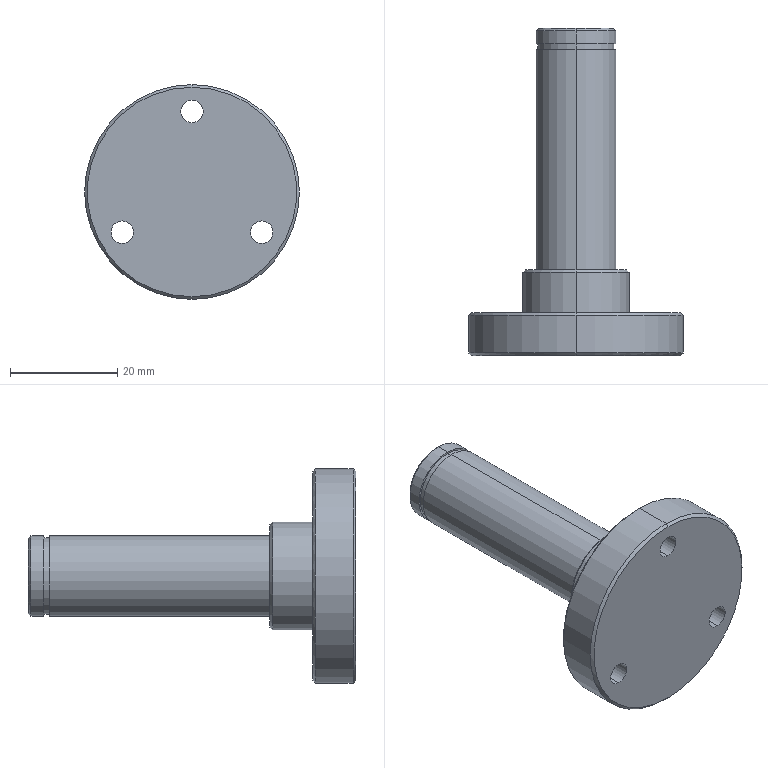Part | SolidWorks | features Chamfer 2, ICE 2, Extrusion 1, HoleWzd 1, RevCut 1 | 1 solid | 30 faces | box 40 x 61 x 40 mm | volume 20124 mm3 | cylinder 16 | cone 8 | plane 6 | commonest cylinder face diameters 4.2 x6 15 x4 14.3 x2 20 x2 40 x2
STEP:
#1=CARTESIAN_POINT('',(0.,4.,19.5));
#2=VERTEX_POINT('',#1);
#3=CARTESIAN_POINT('',(0.,4.,-19.5));
#4=VERTEX_POINT('',#3);
#5=CARTESIAN_POINT('',(0.,4.,0.));
#6=DIRECTION('',(0.,1.,0.));
#7=DIRECTION('',(0.,0.,1.));
#8=AXIS2_PLACEMENT_3D('',#5,#6,#7);
#9=CIRCLE('',#8,19.5);
#10=EDGE_CURVE('',#2,#4,#9,.T.);
#11=ORIENTED_EDGE('',*,*,#10,.F.);
#12=CARTESIAN_POINT('',(0.,3.5,20.));
#13=VERTEX_POINT('',#12);
#14=CARTESIAN_POINT('',(0.,4.,19.5));
#15=DIRECTION('',(0.,-0.7071,0.7071));
#16=VECTOR('',#15,1000.);
#17=LINE('',#14,#16);
#18=EDGE_CURVE('',#2,#13,#17,.T.);
#19=ORIENTED_EDGE('',*,*,#18,.T.);
#20=CARTESIAN_POINT('',(0.,3.5,-20.));
#21=VERTEX_POINT('',#20);
#22=CARTESIAN_POINT('',(0.,3.5,0.));
#23=DIRECTION('',(0.,-1.,0.));
#24=DIRECTION('',(0.,0.,1.));
#25=AXIS2_PLACEMENT_3D('',#22,#23,#24);
#26=CIRCLE('',#25,20.);
#27=EDGE_CURVE('',#21,#13,#26,.T.);
#28=ORIENTED_EDGE('',*,*,#27,.F.);
#29=CARTESIAN_POINT('',(0.,4.,-19.5));
#30=DIRECTION('',(0.,-0.7071,-0.7071));
#31=VECTOR('',#30,1000.);
#32=LINE('',#29,#31);
#33=EDGE_CURVE('',#4,#21,#32,.T.);
#34=ORIENTED_EDGE('',*,*,#33,.F.);
#35=EDGE_LOOP('',(#11,#19,#28,#34));
#36=FACE_OUTER_BOUND('',#35,.T.);
#37=CARTESIAN_POINT('',(0.,4.,0.));
#38=DIRECTION('',(0.,-1.,0.));
#39=DIRECTION('',(0.,0.,-1.));
#40=AXIS2_PLACEMENT_3D('',#37,#38,#39);
#41=CONICAL_SURFACE('',#40,19.5,0.7854);
#42=ADVANCED_FACE('',(#36),#41,.T.);
#43=CARTESIAN_POINT('',(0.,-4.,-19.5));
#44=VERTEX_POINT('',#43);
#45=CARTESIAN_POINT('',(0.,-4.,19.5));
#46=VERTEX_POINT('',#45);
#47=CARTESIAN_POINT('',(0.,-4.,0.));
#48=DIRECTION('',(0.,-1.,0.));
#49=DIRECTION('',(0.,0.,1.));
#50=AXIS2_PLACEMENT_3D('',#47,#48,#49);
#51=CIRCLE('',#50,19.5);
#52=EDGE_CURVE('',#44,#46,#51,.T.);
#53=ORIENTED_EDGE('',*,*,#52,.F.);
#54=CARTESIAN_POINT('',(0.,-3.5,-20.));
#55=VERTEX_POINT('',#54);
#56=CARTESIAN_POINT('',(0.,-3.5,-20.));
#57=DIRECTION('',(0.,0.7071,-0.7071));
#58=VECTOR('',#57,1000.);
#59=LINE('',#56,#58);
#60=EDGE_CURVE('',#44,#55,#59,.T.);
#61=ORIENTED_EDGE('',*,*,#60,.T.);
#62=CARTESIAN_POINT('',(0.,-3.5,20.));
#63=VERTEX_POINT('',#62);
#64=CARTESIAN_POINT('',(0.,-3.5,0.));
#65=DIRECTION('',(0.,1.,0.));
#66=DIRECTION('',(0.,0.,1.));
#67=AXIS2_PLACEMENT_3D('',#64,#65,#66);
#68=CIRCLE('',#67,20.);
#69=EDGE_CURVE('',#63,#55,#68,.T.);
#70=ORIENTED_EDGE('',*,*,#69,.F.);
#71=CARTESIAN_POINT('',(0.,-3.5,20.));
#72=DIRECTION('',(0.,0.7071,0.7071));
#73=VECTOR('',#72,1000.);
#74=LINE('',#71,#73);
#75=EDGE_CURVE('',#46,#63,#74,.T.);
#76=ORIENTED_EDGE('',*,*,#75,.F.);
#77=EDGE_LOOP('',(#53,#61,#70,#76));
#78=FACE_OUTER_BOUND('',#77,.T.);
#79=CARTESIAN_POINT('',(0.,-3.5,0.));
#80=DIRECTION('',(0.,1.,0.));
#81=DIRECTION('',(0.,0.,1.));
#82=AXIS2_PLACEMENT_3D('',#79,#80,#81);
#83=CONICAL_SURFACE('',#82,20.,0.7854);
#84=ADVANCED_FACE('',(#78),#83,.T.);
#85=CARTESIAN_POINT('',(0.,12.,9.5));
#86=VERTEX_POINT('',#85);
#87=CARTESIAN_POINT('',(0.,12.,-9.5));
#88=VERTEX_POINT('',#87);
#89=CARTESIAN_POINT('',(0.,12.,0.));
#90=DIRECTION('',(0.,1.,0.));
#91=DIRECTION('',(0.,0.,1.));
#92=AXIS2_PLACEMENT_3D('',#89,#90,#91);
#93=CIRCLE('',#92,9.5);
#94=EDGE_CURVE('',#86,#88,#93,.T.);
#95=ORIENTED_EDGE('',*,*,#94,.F.);
#96=CARTESIAN_POINT('',(0.,11.5,10.));
#97=VERTEX_POINT('',#96);
#98=CARTESIAN_POINT('',(0.,12.,9.5));
#99=DIRECTION('',(0.,-0.7071,0.7071));
#100=VECTOR('',#99,1000.);
#101=LINE('',#98,#100);
#102=EDGE_CURVE('',#86,#97,#101,.T.);
#103=ORIENTED_EDGE('',*,*,#102,.T.);
#104=CARTESIAN_POINT('',(0.,11.5,-10.));
#105=VERTEX_POINT('',#104);
#106=CARTESIAN_POINT('',(0.,11.5,0.));
#107=DIRECTION('',(0.,-1.,0.));
#108=DIRECTION('',(0.,0.,1.));
#109=AXIS2_PLACEMENT_3D('',#106,#107,#108);
#110=CIRCLE('',#109,10.);
#111=EDGE_CURVE('',#105,#97,#110,.T.);
#112=ORIENTED_EDGE('',*,*,#111,.F.);
#113=CARTESIAN_POINT('',(0.,12.,-9.5));
#114=DIRECTION('',(0.,-0.7071,-0.7071));
#115=VECTOR('',#114,1000.);
#116=LINE('',#113,#115);
#117=EDGE_CURVE('',#88,#105,#116,.T.);
#118=ORIENTED_EDGE('',*,*,#117,.F.);
#119=EDGE_LOOP('',(#95,#103,#112,#118));
#120=FACE_OUTER_BOUND('',#119,.T.);
#121=CARTESIAN_POINT('',(0.,12.,0.));
#122=DIRECTION('',(0.,-1.,0.));
#123=DIRECTION('',(0.,0.,-1.));
#124=AXIS2_PLACEMENT_3D('',#121,#122,#123);
#125=CONICAL_SURFACE('',#124,9.5,0.7854);
#126=ADVANCED_FACE('',(#120),#125,.T.);
#127=CARTESIAN_POINT('',(0.,57.,7.));
#128=VERTEX_POINT('',#127);
#129=CARTESIAN_POINT('',(0.,57.,-7.));
#130=VERTEX_POINT('',#129);
#131=CARTESIAN_POINT('',(0.,57.,0.));
#132=DIRECTION('',(0.,1.,0.));
#133=DIRECTION('',(0.,0.,1.));
#134=AXIS2_PLACEMENT_3D('',#131,#132,#133);
#135=CIRCLE('',#134,7.);
#136=EDGE_CURVE('',#128,#130,#135,.T.);
#137=ORIENTED_EDGE('',*,*,#136,.F.);
#138=CARTESIAN_POINT('',(0.,56.5,7.5));
#139=VERTEX_POINT('',#138);
#140=CARTESIAN_POINT('',(0.,57.,7.));
#141=DIRECTION('',(0.,-0.7071,0.7071));
#142=VECTOR('',#141,1000.);
#143=LINE('',#140,#142);
#144=EDGE_CURVE('',#128,#139,#143,.T.);
#145=ORIENTED_EDGE('',*,*,#144,.T.);
#146=CARTESIAN_POINT('',(0.,56.5,-7.5));
#147=VERTEX_POINT('',#146);
#148=CARTESIAN_POINT('',(0.,56.5,0.));
#149=DIRECTION('',(0.,-1.,0.));
#150=DIRECTION('',(0.,0.,1.));
#151=AXIS2_PLACEMENT_3D('',#148,#149,#150);
#152=CIRCLE('',#151,7.5);
#153=EDGE_CURVE('',#147,#139,#152,.T.);
#154=ORIENTED_EDGE('',*,*,#153,.F.);
#155=CARTESIAN_POINT('',(0.,57.,-7.));
#156=DIRECTION('',(0.,-0.7071,-0.7071));
#157=VECTOR('',#156,1000.);
#158=LINE('',#155,#157);
#159=EDGE_CURVE('',#130,#147,#158,.T.);
#160=ORIENTED_EDGE('',*,*,#159,.F.);
#161=EDGE_LOOP('',(#137,#145,#154,#160));
#162=FACE_OUTER_BOUND('',#161,.T.);
#163=CARTESIAN_POINT('',(0.,57.,0.));
#164=DIRECTION('',(0.,-1.,0.));
#165=DIRECTION('',(0.,0.,-1.));
#166=AXIS2_PLACEMENT_3D('',#163,#164,#165);
#167=CONICAL_SURFACE('',#166,7.,0.7854);
#168=ADVANCED_FACE('',(#162),#167,.T.);
#169=CARTESIAN_POINT('',(-12.99,-4.,-9.6));
#170=VERTEX_POINT('',#169);
#171=CARTESIAN_POINT('',(-12.99,-4.,-5.4));
#172=VERTEX_POINT('',#171);
#173=CARTESIAN_POINT('',(-12.99,-4.,-7.5));
#174=DIRECTION('',(0.,1.,0.));
#175=DIRECTION('',(0.,0.,1.));
#176=AXIS2_PLACEMENT_3D('',#173,#174,#175);
#177=CIRCLE('',#176,2.1);
#178=EDGE_CURVE('',#170,#172,#177,.T.);
#179=ORIENTED_EDGE('',*,*,#178,.F.);
#180=CARTESIAN_POINT('',(-12.99,4.,-9.6));
#181=VERTEX_POINT('',#180);
#182=CARTESIAN_POINT('',(-12.99,4.,-9.6));
#183=DIRECTION('',(0.,1.,0.));
#184=VECTOR('',#183,1000.);
#185=LINE('',#182,#184);
#186=EDGE_CURVE('',#170,#181,#185,.T.);
#187=ORIENTED_EDGE('',*,*,#186,.T.);
#188=CARTESIAN_POINT('',(-12.99,4.,-5.4));
#189=VERTEX_POINT('',#188);
#190=CARTESIAN_POINT('',(-12.99,4.,-7.5));
#191=DIRECTION('',(0.,1.,0.));
#192=DIRECTION('',(0.,0.,1.));
#193=AXIS2_PLACEMENT_3D('',#190,#191,#192);
#194=CIRCLE('',#193,2.1);
#195=EDGE_CURVE('',#181,#189,#194,.T.);
#196=ORIENTED_EDGE('',*,*,#195,.T.);
#197=CARTESIAN_POINT('',(-12.99,4.,-5.4));
#198=DIRECTION('',(0.,1.,0.));
#199=VECTOR('',#198,1000.);
#200=LINE('',#197,#199);
#201=EDGE_CURVE('',#172,#189,#200,.T.);
#202=ORIENTED_EDGE('',*,*,#201,.F.);
#203=EDGE_LOOP('',(#179,#187,#196,#202));
#204=FACE_OUTER_BOUND('',#203,.T.);
#205=CARTESIAN_POINT('',(-12.99,4.,-7.5));
#206=DIRECTION('',(0.,1.,0.));
#207=DIRECTION('',(0.,0.,1.));
#208=AXIS2_PLACEMENT_3D('',#205,#206,#207);
#209=CYLINDRICAL_SURFACE('',#208,2.1);
#210=ADVANCED_FACE('',(#204),#209,.F.);
#211=CARTESIAN_POINT('',(12.99,-4.,-9.6));
#212=VERTEX_POINT('',#211);
#213=CARTESIAN_POINT('',(12.99,-4.,-5.4));
#214=VERTEX_POINT('',#213);
#215=CARTESIAN_POINT('',(12.99,-4.,-7.5));
#216=DIRECTION('',(0.,1.,0.));
#217=DIRECTION('',(0.,0.,1.));
#218=AXIS2_PLACEMENT_3D('',#215,#216,#217);
#219=CIRCLE('',#218,2.1);
#220=EDGE_CURVE('',#212,#214,#219,.T.);
#221=ORIENTED_EDGE('',*,*,#220,.F.);
#222=CARTESIAN_POINT('',(12.99,4.,-9.6));
#223=VERTEX_POINT('',#222);
#224=CARTESIAN_POINT('',(12.99,4.,-9.6));
#225=DIRECTION('',(0.,1.,0.));
#226=VECTOR('',#225,1000.);
#227=LINE('',#224,#226);
#228=EDGE_CURVE('',#212,#223,#227,.T.);
#229=ORIENTED_EDGE('',*,*,#228,.T.);
#230=CARTESIAN_POINT('',(12.99,4.,-5.4));
#231=VERTEX_POINT('',#230);
#232=CARTESIAN_POINT('',(12.99,4.,-7.5));
#233=DIRECTION('',(0.,1.,0.));
#234=DIRECTION('',(0.,0.,1.));
#235=AXIS2_PLACEMENT_3D('',#232,#233,#234);
#236=CIRCLE('',#235,2.1);
#237=EDGE_CURVE('',#223,#231,#236,.T.);
#238=ORIENTED_EDGE('',*,*,#237,.T.);
#239=CARTESIAN_POINT('',(12.99,4.,-5.4));
#240=DIRECTION('',(0.,1.,0.));
#241=VECTOR('',#240,1000.);
#242=LINE('',#239,#241);
#243=EDGE_CURVE('',#214,#231,#242,.T.);
#244=ORIENTED_EDGE('',*,*,#243,.F.);
#245=EDGE_LOOP('',(#221,#229,#238,#244));
#246=FACE_OUTER_BOUND('',#245,.T.);
#247=CARTESIAN_POINT('',(12.99,4.,-7.5));
#248=DIRECTION('',(0.,1.,0.));
#249=DIRECTION('',(0.,0.,1.));
#250=AXIS2_PLACEMENT_3D('',#247,#248,#249);
#251=CYLINDRICAL_SURFACE('',#250,2.1);
#252=ADVANCED_FACE('',(#246),#251,.F.);
#253=CARTESIAN_POINT('',(0.,-4.,12.9));
#254=VERTEX_POINT('',#253);
#255=CARTESIAN_POINT('',(0.,-4.,17.1));
#256=VERTEX_POINT('',#255);
#257=CARTESIAN_POINT('',(0.,-4.,15.));
#258=DIRECTION('',(0.,1.,0.));
#259=DIRECTION('',(0.,0.,1.));
#260=AXIS2_PLACEMENT_3D('',#257,#258,#259);
#261=CIRCLE('',#260,2.1);
#262=EDGE_CURVE('',#254,#256,#261,.T.);
#263=ORIENTED_EDGE('',*,*,#262,.F.);
#264=CARTESIAN_POINT('',(0.,4.,12.9));
#265=VERTEX_POINT('',#264);
#266=CARTESIAN_POINT('',(0.,4.,12.9));
#267=DIRECTION('',(0.,1.,0.));
#268=VECTOR('',#267,1000.);
#269=LINE('',#266,#268);
#270=EDGE_CURVE('',#254,#265,#269,.T.);
#271=ORIENTED_EDGE('',*,*,#270,.T.);
#272=CARTESIAN_POINT('',(0.,4.,17.1));
#273=VERTEX_POINT('',#272);
#274=CARTESIAN_POINT('',(0.,4.,15.));
#275=DIRECTION('',(0.,1.,0.));
#276=DIRECTION('',(0.,0.,1.));
#277=AXIS2_PLACEMENT_3D('',#274,#275,#276);
#278=CIRCLE('',#277,2.1);
#279=EDGE_CURVE('',#265,#273,#278,.T.);
#280=ORIENTED_EDGE('',*,*,#279,.T.);
#281=CARTESIAN_POINT('',(0.,4.,17.1));
#282=DIRECTION('',(0.,1.,0.));
#283=VECTOR('',#282,1000.);
#284=LINE('',#281,#283);
#285=EDGE_CURVE('',#256,#273,#284,.T.);
#286=ORIENTED_EDGE('',*,*,#285,.F.);
#287=EDGE_LOOP('',(#263,#271,#280,#286));
#288=FACE_OUTER_BOUND('',#287,.T.);
#289=CARTESIAN_POINT('',(0.,4.,15.));
#290=DIRECTION('',(0.,1.,0.));
#291=DIRECTION('',(0.,0.,1.));
#292=AXIS2_PLACEMENT_3D('',#289,#290,#291);
#293=CYLINDRICAL_SURFACE('',#292,2.1);
#294=ADVANCED_FACE('',(#288),#293,.F.);
#295=ORIENTED_EDGE('',*,*,#153,.T.);
#296=CARTESIAN_POINT('',(0.,54.1,7.5));
#297=VERTEX_POINT('',#296);
#298=CARTESIAN_POINT('',(0.,57.,7.5));
#299=DIRECTION('',(0.,-1.,0.));
#300=VECTOR('',#299,1000.);
#301=LINE('',#298,#300);
#302=EDGE_CURVE('',#139,#297,#301,.T.);
#303=ORIENTED_EDGE('',*,*,#302,.T.);
#304=CARTESIAN_POINT('',(0.,54.1,-7.5));
#305=VERTEX_POINT('',#304);
#306=CARTESIAN_POINT('',(0.,54.1,0.));
#307=DIRECTION('',(0.,-1.,0.));
#308=DIRECTION('',(0.,0.,-1.));
#309=AXIS2_PLACEMENT_3D('',#306,#307,#308);
#310=CIRCLE('',#309,7.5);
#311=EDGE_CURVE('',#305,#297,#310,.T.);
#312=ORIENTED_EDGE('',*,*,#311,.F.);
#313=CARTESIAN_POINT('',(0.,57.,-7.5));
#314=DIRECTION('',(0.,-1.,0.));
#315=VECTOR('',#314,1000.);
#316=LINE('',#313,#315);
#317=EDGE_CURVE('',#147,#305,#316,.T.);
#318=ORIENTED_EDGE('',*,*,#317,.F.);
#319=EDGE_LOOP('',(#295,#303,#312,#318));
#320=FACE_OUTER_BOUND('',#319,.T.);
#321=CARTESIAN_POINT('',(0.,57.,0.));
#322=DIRECTION('',(0.,-1.,0.));
#323=DIRECTION('',(0.,0.,-1.));
#324=AXIS2_PLACEMENT_3D('',#321,#322,#323);
#325=CYLINDRICAL_SURFACE('',#324,7.5);
#326=ADVANCED_FACE('',(#320),#325,.T.);
#327=CARTESIAN_POINT('',(0.,54.1,-7.15));
#328=VERTEX_POINT('',#327);
#329=CARTESIAN_POINT('',(0.,54.1,7.15));
#330=VERTEX_POINT('',#329);
#331=CARTESIAN_POINT('',(0.,54.1,0.));
#332=DIRECTION('',(0.,-1.,0.));
#333=DIRECTION('',(0.,0.,-1.));
#334=AXIS2_PLACEMENT_3D('',#331,#332,#333);
#335=CIRCLE('',#334,7.15);
#336=EDGE_CURVE('',#328,#330,#335,.T.);
#337=ORIENTED_EDGE('',*,*,#336,.T.);
#338=CARTESIAN_POINT('',(0.,53.,7.15));
#339=VERTEX_POINT('',#338);
#340=CARTESIAN_POINT('',(0.,0.,7.15));
#341=DIRECTION('',(0.,-1.,0.));
#342=VECTOR('',#341,1000.);
#343=LINE('',#340,#342);
#344=EDGE_CURVE('',#330,#339,#343,.T.);
#345=ORIENTED_EDGE('',*,*,#344,.T.);
#346=CARTESIAN_POINT('',(0.,53.,-7.15));
#347=VERTEX_POINT('',#346);
#348=CARTESIAN_POINT('',(0.,53.,0.));
#349=DIRECTION('',(0.,-1.,0.));
#350=DIRECTION('',(0.,0.,-1.));
#351=AXIS2_PLACEMENT_3D('',#348,#349,#350);
#352=CIRCLE('',#351,7.15);
#353=EDGE_CURVE('',#347,#339,#352,.T.);
#354=ORIENTED_EDGE('',*,*,#353,.F.);
#355=CARTESIAN_POINT('',(0.,0.,-7.15));
#356=DIRECTION('',(0.,-1.,0.));
#357=VECTOR('',#356,1000.);
#358=LINE('',#355,#357);
#359=EDGE_CURVE('',#328,#347,#358,.T.);
#360=ORIENTED_EDGE('',*,*,#359,.F.);
#361=EDGE_LOOP('',(#337,#345,#354,#360));
#362=FACE_OUTER_BOUND('',#361,.T.);
#363=CARTESIAN_POINT('',(0.,0.,0.));
#364=DIRECTION('',(0.,-1.,0.));
#365=DIRECTION('',(0.,0.,-1.));
#366=AXIS2_PLACEMENT_3D('',#363,#364,#365);
#367=CYLINDRICAL_SURFACE('',#366,7.15);
#368=ADVANCED_FACE('',(#362),#367,.T.);
#369=ORIENTED_EDGE('',*,*,#111,.T.);
#370=CARTESIAN_POINT('',(0.,4.,10.));
#371=VERTEX_POINT('',#370);
#372=CARTESIAN_POINT('',(0.,12.,10.));
#373=DIRECTION('',(0.,-1.,0.));
#374=VECTOR('',#373,1000.);
#375=LINE('',#372,#374);
#376=EDGE_CURVE('',#97,#371,#375,.T.);
#377=ORIENTED_EDGE('',*,*,#376,.T.);
#378=CARTESIAN_POINT('',(0.,4.,-10.));
#379=VERTEX_POINT('',#378);
#380=CARTESIAN_POINT('',(0.,4.,0.));
#381=DIRECTION('',(0.,1.,0.));
#382=DIRECTION('',(0.,0.,1.));
#383=AXIS2_PLACEMENT_3D('',#380,#381,#382);
#384=CIRCLE('',#383,10.);
#385=EDGE_CURVE('',#371,#379,#384,.T.);
#386=ORIENTED_EDGE('',*,*,#385,.T.);
#387=CARTESIAN_POINT('',(0.,12.,-10.));
#388=DIRECTION('',(0.,-1.,0.));
#389=VECTOR('',#388,1000.);
#390=LINE('',#387,#389);
#391=EDGE_CURVE('',#105,#379,#390,.T.);
#392=ORIENTED_EDGE('',*,*,#391,.F.);
#393=EDGE_LOOP('',(#369,#377,#386,#392));
#394=FACE_OUTER_BOUND('',#393,.T.);
#395=CARTESIAN_POINT('',(0.,12.,0.));
#396=DIRECTION('',(0.,-1.,0.));
#397=DIRECTION('',(0.,0.,-1.));
#398=AXIS2_PLACEMENT_3D('',#395,#396,#397);
#399=CYLINDRICAL_SURFACE('',#398,10.);
#400=ADVANCED_FACE('',(#394),#399,.T.);
#401=ORIENTED_EDGE('',*,*,#27,.T.);
#402=CARTESIAN_POINT('',(0.,4.,20.));
#403=DIRECTION('',(0.,-1.,0.));
#404=VECTOR('',#403,1000.);
#405=LINE('',#402,#404);
#406=EDGE_CURVE('',#13,#63,#405,.T.);
#407=ORIENTED_EDGE('',*,*,#406,.T.);
#408=ORIENTED_EDGE('',*,*,#69,.T.);
#409=CARTESIAN_POINT('',(0.,4.,-20.));
#410=DIRECTION('',(0.,-1.,0.));
#411=VECTOR('',#410,1000.);
#412=LINE('',#409,#411);
#413=EDGE_CURVE('',#21,#55,#412,.T.);
#414=ORIENTED_EDGE('',*,*,#413,.F.);
#415=EDGE_LOOP('',(#401,#407,#408,#414));
#416=FACE_OUTER_BOUND('',#415,.T.);
#417=CARTESIAN_POINT('',(0.,4.,0.));
#418=DIRECTION('',(0.,-1.,0.));
#419=DIRECTION('',(0.,0.,-1.));
#420=AXIS2_PLACEMENT_3D('',#417,#418,#419);
#421=CYLINDRICAL_SURFACE('',#420,20.);
#422=ADVANCED_FACE('',(#416),#421,.T.);
#423=CARTESIAN_POINT('',(0.,53.,-7.5));
#424=VERTEX_POINT('',#423);
#425=CARTESIAN_POINT('',(0.,53.,7.5));
#426=VERTEX_POINT('',#425);
#427=CARTESIAN_POINT('',(0.,53.,0.));
#428=DIRECTION('',(0.,-1.,0.));
#429=DIRECTION('',(0.,0.,-1.));
#430=AXIS2_PLACEMENT_3D('',#427,#428,#429);
#431=CIRCLE('',#430,7.5);
#432=EDGE_CURVE('',#424,#426,#431,.T.);
#433=ORIENTED_EDGE('',*,*,#432,.T.);
#434=CARTESIAN_POINT('',(0.,12.,7.5));
#435=VERTEX_POINT('',#434);
#436=CARTESIAN_POINT('',(0.,57.,7.5));
#437=DIRECTION('',(0.,-1.,0.));
#438=VECTOR('',#437,1000.);
#439=LINE('',#436,#438);
#440=EDGE_CURVE('',#426,#435,#439,.T.);
#441=ORIENTED_EDGE('',*,*,#440,.T.);
#442=CARTESIAN_POINT('',(0.,12.,-7.5));
#443=VERTEX_POINT('',#442);
#444=CARTESIAN_POINT('',(0.,12.,0.));
#445=DIRECTION('',(0.,1.,0.));
#446=DIRECTION('',(0.,0.,1.));
#447=AXIS2_PLACEMENT_3D('',#444,#445,#446);
#448=CIRCLE('',#447,7.5);
#449=EDGE_CURVE('',#435,#443,#448,.T.);
#450=ORIENTED_EDGE('',*,*,#449,.T.);
#451=CARTESIAN_POINT('',(0.,57.,-7.5));
#452=DIRECTION('',(0.,-1.,0.));
#453=VECTOR('',#452,1000.);
#454=LINE('',#451,#453);
#455=EDGE_CURVE('',#424,#443,#454,.T.);
#456=ORIENTED_EDGE('',*,*,#455,.F.);
#457=EDGE_LOOP('',(#433,#441,#450,#456));
#458=FACE_OUTER_BOUND('',#457,.T.);
#459=CARTESIAN_POINT('',(0.,57.,0.));
#460=DIRECTION('',(0.,-1.,0.));
#461=DIRECTION('',(0.,0.,-1.));
#462=AXIS2_PLACEMENT_3D('',#459,#460,#461);
#463=CYLINDRICAL_SURFACE('',#462,7.5);
#464=ADVANCED_FACE('',(#458),#463,.T.);
#465=ORIENTED_EDGE('',*,*,#440,.F.);
#466=CARTESIAN_POINT('',(0.,53.,0.));
#467=DIRECTION('',(0.,-1.,0.));
#468=DIRECTION('',(0.,0.,-1.));
#469=AXIS2_PLACEMENT_3D('',#466,#467,#468);
#470=CIRCLE('',#469,7.5);
#471=EDGE_CURVE('',#426,#424,#470,.T.);
#472=ORIENTED_EDGE('',*,*,#471,.T.);
#473=ORIENTED_EDGE('',*,*,#455,.T.);
#474=CARTESIAN_POINT('',(0.,12.,0.));
#475=DIRECTION('',(0.,1.,0.));
#476=DIRECTION('',(0.,0.,1.));
#477=AXIS2_PLACEMENT_3D('',#474,#475,#476);
#478=CIRCLE('',#477,7.5);
#479=EDGE_CURVE('',#443,#435,#478,.T.);
#480=ORIENTED_EDGE('',*,*,#479,.T.);
#481=EDGE_LOOP('',(#465,#472,#473,#480));
#482=FACE_OUTER_BOUND('',#481,.T.);
#483=CARTESIAN_POINT('',(0.,57.,0.));
#484=DIRECTION('',(0.,-1.,0.));
#485=DIRECTION('',(0.,0.,-1.));
#486=AXIS2_PLACEMENT_3D('',#483,#484,#485);
#487=CYLINDRICAL_SURFACE('',#486,7.5);
#488=ADVANCED_FACE('',(#482),#487,.T.);
#489=CARTESIAN_POINT('',(0.,12.,0.));
#490=DIRECTION('',(0.,1.,0.));
#491=DIRECTION('',(0.,0.,1.));
#492=AXIS2_PLACEMENT_3D('',#489,#490,#491);
#493=CIRCLE('',#492,9.5);
#494=EDGE_CURVE('',#88,#86,#493,.T.);
#495=ORIENTED_EDGE('',*,*,#494,.T.);
#496=ORIENTED_EDGE('',*,*,#94,.T.);
#497=EDGE_LOOP('',(#495,#496));
#498=FACE_OUTER_BOUND('',#497,.T.);
#499=ORIENTED_EDGE('',*,*,#479,.F.);
#500=ORIENTED_EDGE('',*,*,#449,.F.);
#501=EDGE_LOOP('',(#499,#500));
#502=FACE_BOUND('',#501,.T.);
#503=CARTESIAN_POINT('',(0.,12.,0.));
#504=DIRECTION('',(0.,1.,0.));
#505=DIRECTION('',(0.,0.,1.));
#506=AXIS2_PLACEMENT_3D('',#503,#504,#505);
#507=PLANE('',#506);
#508=ADVANCED_FACE('',(#498,#502),#507,.T.);
#509=CARTESIAN_POINT('',(0.,4.,0.));
#510=DIRECTION('',(0.,1.,0.));
#511=DIRECTION('',(0.,0.,1.));
#512=AXIS2_PLACEMENT_3D('',#509,#510,#511);
#513=CIRCLE('',#512,19.5);
#514=EDGE_CURVE('',#4,#2,#513,.T.);
#515=ORIENTED_EDGE('',*,*,#514,.T.);
#516=ORIENTED_EDGE('',*,*,#10,.T.);
#517=EDGE_LOOP('',(#515,#516));
#518=FACE_OUTER_BOUND('',#517,.T.);
#519=CARTESIAN_POINT('',(-12.99,4.,-7.5));
#520=DIRECTION('',(0.,1.,0.));
#521=DIRECTION('',(0.,0.,1.));
#522=AXIS2_PLACEMENT_3D('',#519,#520,#521);
#523=CIRCLE('',#522,2.1);
#524=EDGE_CURVE('',#189,#181,#523,.T.);
#525=ORIENTED_EDGE('',*,*,#524,.F.);
#526=ORIENTED_EDGE('',*,*,#195,.F.);
#527=EDGE_LOOP('',(#525,#526));
#528=FACE_BOUND('',#527,.T.);
#529=CARTESIAN_POINT('',(12.99,4.,-7.5));
#530=DIRECTION('',(0.,1.,0.));
#531=DIRECTION('',(0.,0.,1.));
#532=AXIS2_PLACEMENT_3D('',#529,#530,#531);
#533=CIRCLE('',#532,2.1);
#534=EDGE_CURVE('',#231,#223,#533,.T.);
#535=ORIENTED_EDGE('',*,*,#534,.F.);
#536=ORIENTED_EDGE('',*,*,#237,.F.);
#537=EDGE_LOOP('',(#535,#536));
#538=FACE_BOUND('',#537,.T.);
#539=CARTESIAN_POINT('',(0.,4.,15.));
#540=DIRECTION('',(0.,1.,0.));
#541=DIRECTION('',(0.,0.,1.));
#542=AXIS2_PLACEMENT_3D('',#539,#540,#541);
#543=CIRCLE('',#542,2.1);
#544=EDGE_CURVE('',#273,#265,#543,.T.);
#545=ORIENTED_EDGE('',*,*,#544,.F.);
#546=ORIENTED_EDGE('',*,*,#279,.F.);
#547=EDGE_LOOP('',(#545,#546));
#548=FACE_BOUND('',#547,.T.);
#549=CARTESIAN_POINT('',(0.,4.,0.));
#550=DIRECTION('',(0.,1.,0.));
#551=DIRECTION('',(0.,0.,1.));
#552=AXIS2_PLACEMENT_3D('',#549,#550,#551);
#553=CIRCLE('',#552,10.);
#554=EDGE_CURVE('',#379,#371,#553,.T.);
#555=ORIENTED_EDGE('',*,*,#554,.F.);
#556=ORIENTED_EDGE('',*,*,#385,.F.);
#557=EDGE_LOOP('',(#555,#556));
#558=FACE_BOUND('',#557,.T.);
#559=CARTESIAN_POINT('',(0.,4.,0.));
#560=DIRECTION('',(0.,1.,0.));
#561=DIRECTION('',(0.,0.,1.));
#562=AXIS2_PLACEMENT_3D('',#559,#560,#561);
#563=PLANE('',#562);
#564=ADVANCED_FACE('',(#518,#528,#538,#548,#558),#563,.T.);
#565=ORIENTED_EDGE('',*,*,#406,.F.);
#566=CARTESIAN_POINT('',(0.,3.5,0.));
#567=DIRECTION('',(0.,-1.,0.));
#568=DIRECTION('',(0.,0.,1.));
#569=AXIS2_PLACEMENT_3D('',#566,#567,#568);
#570=CIRCLE('',#569,20.);
#571=EDGE_CURVE('',#13,#21,#570,.T.);
#572=ORIENTED_EDGE('',*,*,#571,.T.);
#573=ORIENTED_EDGE('',*,*,#413,.T.);
#574=CARTESIAN_POINT('',(0.,-3.5,0.));
#575=DIRECTION('',(0.,1.,0.));
#576=DIRECTION('',(0.,0.,1.));
#577=AXIS2_PLACEMENT_3D('',#574,#575,#576);
#578=CIRCLE('',#577,20.);
#579=EDGE_CURVE('',#55,#63,#578,.T.);
#580=ORIENTED_EDGE('',*,*,#579,.T.);
#581=EDGE_LOOP('',(#565,#572,#573,#580));
#582=FACE_OUTER_BOUND('',#581,.T.);
#583=CARTESIAN_POINT('',(0.,4.,0.));
#584=DIRECTION('',(0.,-1.,0.));
#585=DIRECTION('',(0.,0.,-1.));
#586=AXIS2_PLACEMENT_3D('',#583,#584,#585);
#587=CYLINDRICAL_SURFACE('',#586,20.);
#588=ADVANCED_FACE('',(#582),#587,.T.);
#589=CARTESIAN_POINT('',(0.,-4.,0.));
#590=DIRECTION('',(0.,-1.,0.));
#591=DIRECTION('',(0.,0.,1.));
#592=AXIS2_PLACEMENT_3D('',#589,#590,#591);
#593=CIRCLE('',#592,19.5);
#594=EDGE_CURVE('',#46,#44,#593,.T.);
#595=ORIENTED_EDGE('',*,*,#594,.T.);
#596=ORIENTED_EDGE('',*,*,#52,.T.);
#597=EDGE_LOOP('',(#595,#596));
#598=FACE_OUTER_BOUND('',#597,.T.);
#599=CARTESIAN_POINT('',(-12.99,-4.,-7.5));
#600=DIRECTION('',(0.,1.,0.));
#601=DIRECTION('',(0.,0.,1.));
#602=AXIS2_PLACEMENT_3D('',#599,#600,#601);
#603=CIRCLE('',#602,2.1);
#604=EDGE_CURVE('',#172,#170,#603,.T.);
#605=ORIENTED_EDGE('',*,*,#604,.T.);
#606=ORIENTED_EDGE('',*,*,#178,.T.);
#607=EDGE_LOOP('',(#605,#606));
#608=FACE_BOUND('',#607,.T.);
#609=CARTESIAN_POINT('',(12.99,-4.,-7.5));
#610=DIRECTION('',(0.,1.,0.));
#611=DIRECTION('',(0.,0.,1.));
#612=AXIS2_PLACEMENT_3D('',#609,#610,#611);
#613=CIRCLE('',#612,2.1);
#614=EDGE_CURVE('',#214,#212,#613,.T.);
#615=ORIENTED_EDGE('',*,*,#614,.T.);
#616=ORIENTED_EDGE('',*,*,#220,.T.);
#617=EDGE_LOOP('',(#615,#616));
#618=FACE_BOUND('',#617,.T.);
#619=CARTESIAN_POINT('',(0.,-4.,15.));
#620=DIRECTION('',(0.,1.,0.));
#621=DIRECTION('',(0.,0.,1.));
#622=AXIS2_PLACEMENT_3D('',#619,#620,#621);
#623=CIRCLE('',#622,2.1);
#624=EDGE_CURVE('',#256,#254,#623,.T.);
#625=ORIENTED_EDGE('',*,*,#624,.T.);
#626=ORIENTED_EDGE('',*,*,#262,.T.);
#627=EDGE_LOOP('',(#625,#626));
#628=FACE_BOUND('',#627,.T.);
#629=CARTESIAN_POINT('',(0.,-4.,0.));
#630=DIRECTION('',(0.,1.,0.));
#631=DIRECTION('',(0.,0.,1.));
#632=AXIS2_PLACEMENT_3D('',#629,#630,#631);
#633=PLANE('',#632);
#634=ADVANCED_FACE('',(#598,#608,#618,#628),#633,.F.);
#635=ORIENTED_EDGE('',*,*,#376,.F.);
#636=CARTESIAN_POINT('',(0.,11.5,0.));
#637=DIRECTION('',(0.,-1.,0.));
#638=DIRECTION('',(0.,0.,1.));
#639=AXIS2_PLACEMENT_3D('',#636,#637,#638);
#640=CIRCLE('',#639,10.);
#641=EDGE_CURVE('',#97,#105,#640,.T.);
#642=ORIENTED_EDGE('',*,*,#641,.T.);
#643=ORIENTED_EDGE('',*,*,#391,.T.);
#644=ORIENTED_EDGE('',*,*,#554,.T.);
#645=EDGE_LOOP('',(#635,#642,#643,#644));
#646=FACE_OUTER_BOUND('',#645,.T.);
#647=CARTESIAN_POINT('',(0.,12.,0.));
#648=DIRECTION('',(0.,-1.,0.));
#649=DIRECTION('',(0.,0.,-1.));
#650=AXIS2_PLACEMENT_3D('',#647,#648,#649);
#651=CYLINDRICAL_SURFACE('',#650,10.);
#652=ADVANCED_FACE('',(#646),#651,.T.);
#653=ORIENTED_EDGE('',*,*,#432,.F.);
#654=ORIENTED_EDGE('',*,*,#471,.F.);
#655=EDGE_LOOP('',(#653,#654));
#656=FACE_OUTER_BOUND('',#655,.T.);
#657=ORIENTED_EDGE('',*,*,#353,.T.);
#658=CARTESIAN_POINT('',(0.,53.,0.));
#659=DIRECTION('',(0.,-1.,0.));
#660=DIRECTION('',(0.,0.,-1.));
#661=AXIS2_PLACEMENT_3D('',#658,#659,#660);
#662=CIRCLE('',#661,7.15);
#663=EDGE_CURVE('',#339,#347,#662,.T.);
#664=ORIENTED_EDGE('',*,*,#663,.T.);
#665=EDGE_LOOP('',(#657,#664));
#666=FACE_BOUND('',#665,.T.);
#667=CARTESIAN_POINT('',(0.,53.,-7.5));
#668=DIRECTION('',(0.,-1.,0.));
#669=DIRECTION('',(0.,0.,-1.));
#670=AXIS2_PLACEMENT_3D('',#667,#668,#669);
#671=PLANE('',#670);
#672=ADVANCED_FACE('',(#656,#666),#671,.F.);
#673=ORIENTED_EDGE('',*,*,#344,.F.);
#674=CARTESIAN_POINT('',(0.,54.1,0.));
#675=DIRECTION('',(0.,-1.,0.));
#676=DIRECTION('',(0.,0.,-1.));
#677=AXIS2_PLACEMENT_3D('',#674,#675,#676);
#678=CIRCLE('',#677,7.15);
#679=EDGE_CURVE('',#330,#328,#678,.T.);
#680=ORIENTED_EDGE('',*,*,#679,.T.);
#681=ORIENTED_EDGE('',*,*,#359,.T.);
#682=ORIENTED_EDGE('',*,*,#663,.F.);
#683=EDGE_LOOP('',(#673,#680,#681,#682));
#684=FACE_OUTER_BOUND('',#683,.T.);
#685=CARTESIAN_POINT('',(0.,0.,0.));
#686=DIRECTION('',(0.,-1.,0.));
#687=DIRECTION('',(0.,0.,-1.));
#688=AXIS2_PLACEMENT_3D('',#685,#686,#687);
#689=CYLINDRICAL_SURFACE('',#688,7.15);
#690=ADVANCED_FACE('',(#684),#689,.T.);
#691=ORIENTED_EDGE('',*,*,#336,.F.);
#692=ORIENTED_EDGE('',*,*,#679,.F.);
#693=EDGE_LOOP('',(#691,#692));
#694=FACE_BOUND('',#693,.T.);
#695=ORIENTED_EDGE('',*,*,#311,.T.);
#696=CARTESIAN_POINT('',(0.,54.1,0.));
#697=DIRECTION('',(0.,-1.,0.));
#698=DIRECTION('',(0.,0.,-1.));
#699=AXIS2_PLACEMENT_3D('',#696,#697,#698);
#700=CIRCLE('',#699,7.5);
#701=EDGE_CURVE('',#297,#305,#700,.T.);
#702=ORIENTED_EDGE('',*,*,#701,.T.);
#703=EDGE_LOOP('',(#695,#702));
#704=FACE_OUTER_BOUND('',#703,.T.);
#705=CARTESIAN_POINT('',(0.,54.1,-7.5));
#706=DIRECTION('',(0.,1.,0.));
#707=DIRECTION('',(0.,0.,1.));
#708=AXIS2_PLACEMENT_3D('',#705,#706,#707);
#709=PLANE('',#708);
#710=ADVANCED_FACE('',(#694,#704),#709,.F.);
#711=CARTESIAN_POINT('',(0.,57.,0.));
#712=DIRECTION('',(0.,1.,0.));
#713=DIRECTION('',(0.,0.,1.));
#714=AXIS2_PLACEMENT_3D('',#711,#712,#713);
#715=CIRCLE('',#714,7.);
#716=EDGE_CURVE('',#130,#128,#715,.T.);
#717=ORIENTED_EDGE('',*,*,#716,.T.);
#718=ORIENTED_EDGE('',*,*,#136,.T.);
#719=EDGE_LOOP('',(#717,#718));
#720=FACE_OUTER_BOUND('',#719,.T.);
#721=CARTESIAN_POINT('',(0.,57.,0.));
#722=DIRECTION('',(0.,1.,0.));
#723=DIRECTION('',(0.,0.,1.));
#724=AXIS2_PLACEMENT_3D('',#721,#722,#723);
#725=PLANE('',#724);
#726=ADVANCED_FACE('',(#720),#725,.T.);
#727=ORIENTED_EDGE('',*,*,#302,.F.);
#728=CARTESIAN_POINT('',(0.,56.5,0.));
#729=DIRECTION('',(0.,-1.,0.));
#730=DIRECTION('',(0.,0.,1.));
#731=AXIS2_PLACEMENT_3D('',#728,#729,#730);
#732=CIRCLE('',#731,7.5);
#733=EDGE_CURVE('',#139,#147,#732,.T.);
#734=ORIENTED_EDGE('',*,*,#733,.T.);
#735=ORIENTED_EDGE('',*,*,#317,.T.);
#736=ORIENTED_EDGE('',*,*,#701,.F.);
#737=EDGE_LOOP('',(#727,#734,#735,#736));
#738=FACE_OUTER_BOUND('',#737,.T.);
#739=CARTESIAN_POINT('',(0.,57.,0.));
#740=DIRECTION('',(0.,-1.,0.));
#741=DIRECTION('',(0.,0.,-1.));
#742=AXIS2_PLACEMENT_3D('',#739,#740,#741);
#743=CYLINDRICAL_SURFACE('',#742,7.5);
#744=ADVANCED_FACE('',(#738),#743,.T.);
#745=ORIENTED_EDGE('',*,*,#270,.F.);
#746=ORIENTED_EDGE('',*,*,#624,.F.);
#747=ORIENTED_EDGE('',*,*,#285,.T.);
#748=ORIENTED_EDGE('',*,*,#544,.T.);
#749=EDGE_LOOP('',(#745,#746,#747,#748));
#750=FACE_OUTER_BOUND('',#749,.T.);
#751=CARTESIAN_POINT('',(0.,4.,15.));
#752=DIRECTION('',(0.,1.,0.));
#753=DIRECTION('',(0.,0.,1.));
#754=AXIS2_PLACEMENT_3D('',#751,#752,#753);
#755=CYLINDRICAL_SURFACE('',#754,2.1);
#756=ADVANCED_FACE('',(#750),#755,.F.);
#757=ORIENTED_EDGE('',*,*,#228,.F.);
#758=ORIENTED_EDGE('',*,*,#614,.F.);
#759=ORIENTED_EDGE('',*,*,#243,.T.);
#760=ORIENTED_EDGE('',*,*,#534,.T.);
#761=EDGE_LOOP('',(#757,#758,#759,#760));
#762=FACE_OUTER_BOUND('',#761,.T.);
#763=CARTESIAN_POINT('',(12.99,4.,-7.5));
#764=DIRECTION('',(0.,1.,0.));
#765=DIRECTION('',(0.,0.,1.));
#766=AXIS2_PLACEMENT_3D('',#763,#764,#765);
#767=CYLINDRICAL_SURFACE('',#766,2.1);
#768=ADVANCED_FACE('',(#762),#767,.F.);
#769=ORIENTED_EDGE('',*,*,#186,.F.);
#770=ORIENTED_EDGE('',*,*,#604,.F.);
#771=ORIENTED_EDGE('',*,*,#201,.T.);
#772=ORIENTED_EDGE('',*,*,#524,.T.);
#773=EDGE_LOOP('',(#769,#770,#771,#772));
#774=FACE_OUTER_BOUND('',#773,.T.);
#775=CARTESIAN_POINT('',(-12.99,4.,-7.5));
#776=DIRECTION('',(0.,1.,0.));
#777=DIRECTION('',(0.,0.,1.));
#778=AXIS2_PLACEMENT_3D('',#775,#776,#777);
#779=CYLINDRICAL_SURFACE('',#778,2.1);
#780=ADVANCED_FACE('',(#774),#779,.F.);
#781=ORIENTED_EDGE('',*,*,#144,.F.);
#782=ORIENTED_EDGE('',*,*,#716,.F.);
#783=ORIENTED_EDGE('',*,*,#159,.T.);
#784=ORIENTED_EDGE('',*,*,#733,.F.);
#785=EDGE_LOOP('',(#781,#782,#783,#784));
#786=FACE_OUTER_BOUND('',#785,.T.);
#787=CARTESIAN_POINT('',(0.,57.,0.));
#788=DIRECTION('',(0.,-1.,0.));
#789=DIRECTION('',(0.,0.,-1.));
#790=AXIS2_PLACEMENT_3D('',#787,#788,#789);
#791=CONICAL_SURFACE('',#790,7.,0.7854);
#792=ADVANCED_FACE('',(#786),#791,.T.);
#793=ORIENTED_EDGE('',*,*,#102,.F.);
#794=ORIENTED_EDGE('',*,*,#494,.F.);
#795=ORIENTED_EDGE('',*,*,#117,.T.);
#796=ORIENTED_EDGE('',*,*,#641,.F.);
#797=EDGE_LOOP('',(#793,#794,#795,#796));
#798=FACE_OUTER_BOUND('',#797,.T.);
#799=CARTESIAN_POINT('',(0.,12.,0.));
#800=DIRECTION('',(0.,-1.,0.));
#801=DIRECTION('',(0.,0.,-1.));
#802=AXIS2_PLACEMENT_3D('',#799,#800,#801);
#803=CONICAL_SURFACE('',#802,9.5,0.7854);
#804=ADVANCED_FACE('',(#798),#803,.T.);
#805=ORIENTED_EDGE('',*,*,#60,.F.);
#806=ORIENTED_EDGE('',*,*,#594,.F.);
#807=ORIENTED_EDGE('',*,*,#75,.T.);
#808=ORIENTED_EDGE('',*,*,#579,.F.);
#809=EDGE_LOOP('',(#805,#806,#807,#808));
#810=FACE_OUTER_BOUND('',#809,.T.);
#811=CARTESIAN_POINT('',(0.,-3.5,0.));
#812=DIRECTION('',(0.,1.,0.));
#813=DIRECTION('',(0.,0.,1.));
#814=AXIS2_PLACEMENT_3D('',#811,#812,#813);
#815=CONICAL_SURFACE('',#814,20.,0.7854);
#816=ADVANCED_FACE('',(#810),#815,.T.);
#817=ORIENTED_EDGE('',*,*,#18,.F.);
#818=ORIENTED_EDGE('',*,*,#514,.F.);
#819=ORIENTED_EDGE('',*,*,#33,.T.);
#820=ORIENTED_EDGE('',*,*,#571,.F.);
#821=EDGE_LOOP('',(#817,#818,#819,#820));
#822=FACE_OUTER_BOUND('',#821,.T.);
#823=CARTESIAN_POINT('',(0.,4.,0.));
#824=DIRECTION('',(0.,-1.,0.));
#825=DIRECTION('',(0.,0.,-1.));
#826=AXIS2_PLACEMENT_3D('',#823,#824,#825);
#827=CONICAL_SURFACE('',#826,19.5,0.7854);
#828=ADVANCED_FACE('',(#822),#827,.T.);
#829=CLOSED_SHELL('',(#42,#84,#126,#168,#210,#252,#294,#326,#368,#400,#422,#464,#488,#508,#564,#588,#634,#652,#672,#690,#710,#726,#744,#756,#768,#780,#792,#804,#816,#828));
#830=MANIFOLD_SOLID_BREP('',#829);
#831=CARTESIAN_POINT('',(0.,0.,0.));
#832=DIRECTION('',(0.,0.,1.));
#833=DIRECTION('',(1.,0.,0.));
#834=AXIS2_PLACEMENT_3D('',#831,#832,#833);
#835=(LENGTH_UNIT()NAMED_UNIT(*)SI_UNIT(.MILLI.,.METRE.));
#836=UNCERTAINTY_MEASURE_WITH_UNIT(LENGTH_MEASURE(0.00001),#835,'','');
#837=(NAMED_UNIT(*)PLANE_ANGLE_UNIT()SI_UNIT($,.RADIAN.));
#838=(NAMED_UNIT(*)SI_UNIT($,.STERADIAN.)SOLID_ANGLE_UNIT());
#839=(GEOMETRIC_REPRESENTATION_CONTEXT(3)GLOBAL_UNCERTAINTY_ASSIGNED_CONTEXT((#836))GLOBAL_UNIT_ASSIGNED_CONTEXT((#835,#837,#838))REPRESENTATION_CONTEXT('',''));
#840=ADVANCED_BREP_SHAPE_REPRESENTATION('',(#830,#834),#839);